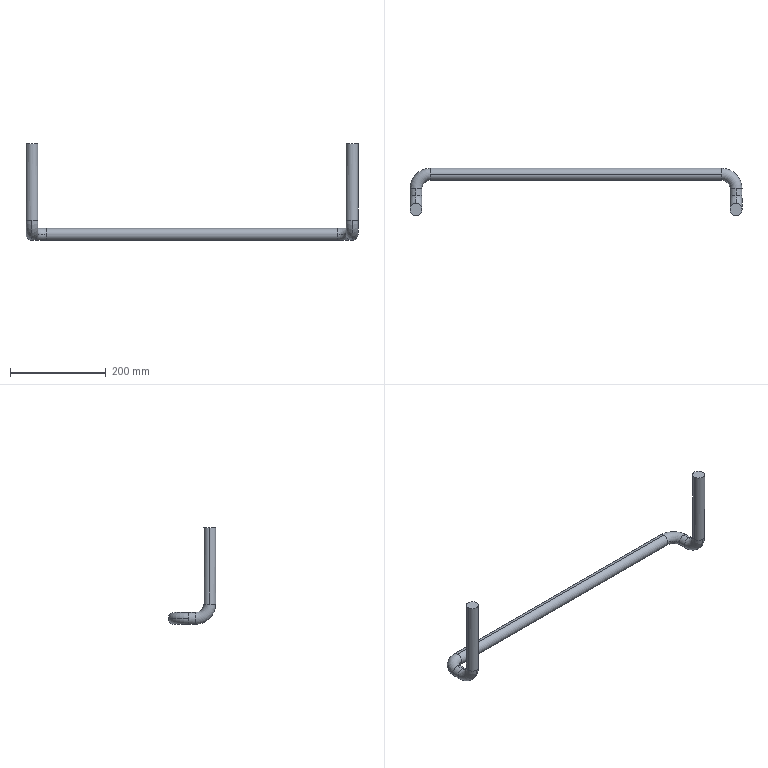Part | SolidWorks | features 3DProfileFeature 2, Sweep 1 | 1 solid | 20 faces | box 695 x 99.162 x 202.5 mm | volume 562944 mm3 | cylinder 10 | torus 8 | plane 2 | commonest cylinder face diameters 25 x10
STEP:
#1=CARTESIAN_POINT('',(-335.,-44.162,-12.5));
#2=VERTEX_POINT('',#1);
#3=CARTESIAN_POINT('',(-335.,-44.162,12.5));
#4=VERTEX_POINT('',#3);
#5=CARTESIAN_POINT('',(-335.,-44.162,0.));
#6=DIRECTION('',(0.,1.,0.));
#7=DIRECTION('',(-1.,0.,0.));
#8=AXIS2_PLACEMENT_3D('',#5,#6,#7);
#9=CIRCLE('',#8,12.5);
#10=EDGE_CURVE('',#2,#4,#9,.T.);
#11=ORIENTED_EDGE('',*,*,#10,.F.);
#12=CARTESIAN_POINT('',(-335.,-86.662,30.));
#13=VERTEX_POINT('',#12);
#14=CARTESIAN_POINT('',(-335.,-44.162,30.));
#15=DIRECTION('',(-1.,0.,0.));
#16=DIRECTION('',(0.,0.,1.));
#17=AXIS2_PLACEMENT_3D('',#14,#15,#16);
#18=CIRCLE('',#17,42.5);
#19=EDGE_CURVE('',#2,#13,#18,.T.);
#20=ORIENTED_EDGE('',*,*,#19,.T.);
#21=CARTESIAN_POINT('',(-347.5,-74.162,30.));
#22=VERTEX_POINT('',#21);
#23=CARTESIAN_POINT('',(-335.,-74.162,30.));
#24=DIRECTION('',(0.,0.,-1.));
#25=DIRECTION('',(-1.,0.,0.));
#26=AXIS2_PLACEMENT_3D('',#23,#24,#25);
#27=CIRCLE('',#26,12.5);
#28=EDGE_CURVE('',#13,#22,#27,.T.);
#29=ORIENTED_EDGE('',*,*,#28,.T.);
#30=CARTESIAN_POINT('',(-335.,-61.662,30.));
#31=VERTEX_POINT('',#30);
#32=CARTESIAN_POINT('',(-335.,-74.162,30.));
#33=DIRECTION('',(0.,0.,-1.));
#34=DIRECTION('',(-1.,0.,0.));
#35=AXIS2_PLACEMENT_3D('',#32,#33,#34);
#36=CIRCLE('',#35,12.5);
#37=EDGE_CURVE('',#22,#31,#36,.T.);
#38=ORIENTED_EDGE('',*,*,#37,.T.);
#39=CARTESIAN_POINT('',(-335.,-44.162,30.));
#40=DIRECTION('',(-1.,0.,0.));
#41=DIRECTION('',(0.,0.,1.));
#42=AXIS2_PLACEMENT_3D('',#39,#40,#41);
#43=CIRCLE('',#42,17.5);
#44=EDGE_CURVE('',#4,#31,#43,.T.);
#45=ORIENTED_EDGE('',*,*,#44,.F.);
#46=EDGE_LOOP('',(#11,#20,#29,#38,#45));
#47=FACE_OUTER_BOUND('',#46,.T.);
#48=CARTESIAN_POINT('',(-335.,-44.162,30.));
#49=DIRECTION('',(-1.,0.,0.));
#50=DIRECTION('',(0.,0.,1.));
#51=AXIS2_PLACEMENT_3D('',#48,#49,#50);
#52=TOROIDAL_SURFACE('',#51,30.,12.5);
#53=ADVANCED_FACE('',(#47),#52,.T.);
#54=CARTESIAN_POINT('',(-305.,12.5,0.));
#55=VERTEX_POINT('',#54);
#56=CARTESIAN_POINT('',(-305.,0.,12.5));
#57=VERTEX_POINT('',#56);
#58=CARTESIAN_POINT('',(-305.,0.,0.));
#59=DIRECTION('',(1.,0.,0.));
#60=DIRECTION('',(0.,1.,0.));
#61=AXIS2_PLACEMENT_3D('',#58,#59,#60);
#62=CIRCLE('',#61,12.5);
#63=EDGE_CURVE('',#55,#57,#62,.T.);
#64=ORIENTED_EDGE('',*,*,#63,.F.);
#65=CARTESIAN_POINT('',(-347.5,-30.,0.));
#66=VERTEX_POINT('',#65);
#67=CARTESIAN_POINT('',(-305.,-30.,0.));
#68=DIRECTION('',(0.,0.,1.));
#69=DIRECTION('',(1.,0.,0.));
#70=AXIS2_PLACEMENT_3D('',#67,#68,#69);
#71=CIRCLE('',#70,42.5);
#72=EDGE_CURVE('',#55,#66,#71,.T.);
#73=ORIENTED_EDGE('',*,*,#72,.T.);
#74=CARTESIAN_POINT('',(-335.,-30.,12.5));
#75=VERTEX_POINT('',#74);
#76=CARTESIAN_POINT('',(-335.,-30.,0.));
#77=DIRECTION('',(0.,1.,0.));
#78=DIRECTION('',(-1.,0.,0.));
#79=AXIS2_PLACEMENT_3D('',#76,#77,#78);
#80=CIRCLE('',#79,12.5);
#81=EDGE_CURVE('',#66,#75,#80,.T.);
#82=ORIENTED_EDGE('',*,*,#81,.T.);
#83=CARTESIAN_POINT('',(-322.5,-30.,0.));
#84=VERTEX_POINT('',#83);
#85=CARTESIAN_POINT('',(-335.,-30.,0.));
#86=DIRECTION('',(0.,1.,0.));
#87=DIRECTION('',(-1.,0.,0.));
#88=AXIS2_PLACEMENT_3D('',#85,#86,#87);
#89=CIRCLE('',#88,12.5);
#90=EDGE_CURVE('',#75,#84,#89,.T.);
#91=ORIENTED_EDGE('',*,*,#90,.T.);
#92=CARTESIAN_POINT('',(-305.,-12.5,0.));
#93=VERTEX_POINT('',#92);
#94=CARTESIAN_POINT('',(-305.,-30.,0.));
#95=DIRECTION('',(0.,0.,1.));
#96=DIRECTION('',(1.,0.,0.));
#97=AXIS2_PLACEMENT_3D('',#94,#95,#96);
#98=CIRCLE('',#97,17.5);
#99=EDGE_CURVE('',#93,#84,#98,.T.);
#100=ORIENTED_EDGE('',*,*,#99,.F.);
#101=CARTESIAN_POINT('',(-305.,0.,0.));
#102=DIRECTION('',(1.,0.,0.));
#103=DIRECTION('',(0.,1.,0.));
#104=AXIS2_PLACEMENT_3D('',#101,#102,#103);
#105=CIRCLE('',#104,12.5);
#106=EDGE_CURVE('',#57,#93,#105,.T.);
#107=ORIENTED_EDGE('',*,*,#106,.F.);
#108=EDGE_LOOP('',(#64,#73,#82,#91,#100,#107));
#109=FACE_OUTER_BOUND('',#108,.T.);
#110=CARTESIAN_POINT('',(-305.,-30.,0.));
#111=DIRECTION('',(0.,0.,1.));
#112=DIRECTION('',(1.,0.,0.));
#113=AXIS2_PLACEMENT_3D('',#110,#111,#112);
#114=TOROIDAL_SURFACE('',#113,30.,12.5);
#115=ADVANCED_FACE('',(#109),#114,.T.);
#116=CARTESIAN_POINT('',(347.5,-30.,0.));
#117=VERTEX_POINT('',#116);
#118=CARTESIAN_POINT('',(335.,-30.,12.5));
#119=VERTEX_POINT('',#118);
#120=CARTESIAN_POINT('',(335.,-30.,0.));
#121=DIRECTION('',(0.,-1.,0.));
#122=DIRECTION('',(1.,0.,0.));
#123=AXIS2_PLACEMENT_3D('',#120,#121,#122);
#124=CIRCLE('',#123,12.5);
#125=EDGE_CURVE('',#117,#119,#124,.T.);
#126=ORIENTED_EDGE('',*,*,#125,.F.);
#127=CARTESIAN_POINT('',(305.,12.5,0.));
#128=VERTEX_POINT('',#127);
#129=CARTESIAN_POINT('',(305.,-30.,0.));
#130=DIRECTION('',(0.,0.,1.));
#131=DIRECTION('',(1.,0.,0.));
#132=AXIS2_PLACEMENT_3D('',#129,#130,#131);
#133=CIRCLE('',#132,42.5);
#134=EDGE_CURVE('',#117,#128,#133,.T.);
#135=ORIENTED_EDGE('',*,*,#134,.T.);
#136=CARTESIAN_POINT('',(305.,0.,12.5));
#137=VERTEX_POINT('',#136);
#138=CARTESIAN_POINT('',(305.,0.,0.));
#139=DIRECTION('',(1.,0.,0.));
#140=DIRECTION('',(0.,1.,0.));
#141=AXIS2_PLACEMENT_3D('',#138,#139,#140);
#142=CIRCLE('',#141,12.5);
#143=EDGE_CURVE('',#128,#137,#142,.T.);
#144=ORIENTED_EDGE('',*,*,#143,.T.);
#145=CARTESIAN_POINT('',(305.,-12.5,0.));
#146=VERTEX_POINT('',#145);
#147=CARTESIAN_POINT('',(305.,0.,0.));
#148=DIRECTION('',(1.,0.,0.));
#149=DIRECTION('',(0.,1.,0.));
#150=AXIS2_PLACEMENT_3D('',#147,#148,#149);
#151=CIRCLE('',#150,12.5);
#152=EDGE_CURVE('',#137,#146,#151,.T.);
#153=ORIENTED_EDGE('',*,*,#152,.T.);
#154=CARTESIAN_POINT('',(322.5,-30.,0.));
#155=VERTEX_POINT('',#154);
#156=CARTESIAN_POINT('',(305.,-30.,0.));
#157=DIRECTION('',(0.,0.,1.));
#158=DIRECTION('',(1.,0.,0.));
#159=AXIS2_PLACEMENT_3D('',#156,#157,#158);
#160=CIRCLE('',#159,17.5);
#161=EDGE_CURVE('',#155,#146,#160,.T.);
#162=ORIENTED_EDGE('',*,*,#161,.F.);
#163=CARTESIAN_POINT('',(335.,-30.,0.));
#164=DIRECTION('',(0.,-1.,0.));
#165=DIRECTION('',(1.,0.,0.));
#166=AXIS2_PLACEMENT_3D('',#163,#164,#165);
#167=CIRCLE('',#166,12.5);
#168=EDGE_CURVE('',#119,#155,#167,.T.);
#169=ORIENTED_EDGE('',*,*,#168,.F.);
#170=EDGE_LOOP('',(#126,#135,#144,#153,#162,#169));
#171=FACE_OUTER_BOUND('',#170,.T.);
#172=CARTESIAN_POINT('',(305.,-30.,0.));
#173=DIRECTION('',(0.,0.,1.));
#174=DIRECTION('',(1.,0.,0.));
#175=AXIS2_PLACEMENT_3D('',#172,#173,#174);
#176=TOROIDAL_SURFACE('',#175,30.,12.5);
#177=ADVANCED_FACE('',(#171),#176,.T.);
#178=CARTESIAN_POINT('',(335.,-86.662,30.));
#179=VERTEX_POINT('',#178);
#180=CARTESIAN_POINT('',(347.5,-74.162,30.));
#181=VERTEX_POINT('',#180);
#182=CARTESIAN_POINT('',(335.,-74.162,30.));
#183=DIRECTION('',(0.,0.,1.));
#184=DIRECTION('',(1.,0.,0.));
#185=AXIS2_PLACEMENT_3D('',#182,#183,#184);
#186=CIRCLE('',#185,12.5);
#187=EDGE_CURVE('',#179,#181,#186,.T.);
#188=ORIENTED_EDGE('',*,*,#187,.F.);
#189=CARTESIAN_POINT('',(335.,-44.162,-12.5));
#190=VERTEX_POINT('',#189);
#191=CARTESIAN_POINT('',(335.,-44.162,30.));
#192=DIRECTION('',(1.,0.,0.));
#193=DIRECTION('',(0.,0.,-1.));
#194=AXIS2_PLACEMENT_3D('',#191,#192,#193);
#195=CIRCLE('',#194,42.5);
#196=EDGE_CURVE('',#179,#190,#195,.T.);
#197=ORIENTED_EDGE('',*,*,#196,.T.);
#198=CARTESIAN_POINT('',(335.,-44.162,12.5));
#199=VERTEX_POINT('',#198);
#200=CARTESIAN_POINT('',(335.,-44.162,0.));
#201=DIRECTION('',(0.,-1.,0.));
#202=DIRECTION('',(1.,0.,0.));
#203=AXIS2_PLACEMENT_3D('',#200,#201,#202);
#204=CIRCLE('',#203,12.5);
#205=EDGE_CURVE('',#190,#199,#204,.T.);
#206=ORIENTED_EDGE('',*,*,#205,.T.);
#207=CARTESIAN_POINT('',(335.,-61.662,30.));
#208=VERTEX_POINT('',#207);
#209=CARTESIAN_POINT('',(335.,-44.162,30.));
#210=DIRECTION('',(1.,0.,0.));
#211=DIRECTION('',(0.,0.,-1.));
#212=AXIS2_PLACEMENT_3D('',#209,#210,#211);
#213=CIRCLE('',#212,17.5);
#214=EDGE_CURVE('',#208,#199,#213,.T.);
#215=ORIENTED_EDGE('',*,*,#214,.F.);
#216=CARTESIAN_POINT('',(335.,-74.162,30.));
#217=DIRECTION('',(0.,0.,1.));
#218=DIRECTION('',(1.,0.,0.));
#219=AXIS2_PLACEMENT_3D('',#216,#217,#218);
#220=CIRCLE('',#219,12.5);
#221=EDGE_CURVE('',#181,#208,#220,.T.);
#222=ORIENTED_EDGE('',*,*,#221,.F.);
#223=EDGE_LOOP('',(#188,#197,#206,#215,#222));
#224=FACE_OUTER_BOUND('',#223,.T.);
#225=CARTESIAN_POINT('',(335.,-44.162,30.));
#226=DIRECTION('',(1.,0.,0.));
#227=DIRECTION('',(0.,0.,-1.));
#228=AXIS2_PLACEMENT_3D('',#225,#226,#227);
#229=TOROIDAL_SURFACE('',#228,30.,12.5);
#230=ADVANCED_FACE('',(#224),#229,.T.);
#231=ORIENTED_EDGE('',*,*,#37,.F.);
#232=CARTESIAN_POINT('',(-347.5,-74.162,190.));
#233=VERTEX_POINT('',#232);
#234=CARTESIAN_POINT('',(-347.5,-74.162,30.));
#235=DIRECTION('',(0.,0.,1.));
#236=VECTOR('',#235,1000.);
#237=LINE('',#234,#236);
#238=EDGE_CURVE('',#22,#233,#237,.T.);
#239=ORIENTED_EDGE('',*,*,#238,.T.);
#240=CARTESIAN_POINT('',(-322.5,-74.162,190.));
#241=VERTEX_POINT('',#240);
#242=CARTESIAN_POINT('',(-335.,-74.162,190.));
#243=DIRECTION('',(0.,0.,-1.));
#244=DIRECTION('',(-1.,0.,0.));
#245=AXIS2_PLACEMENT_3D('',#242,#243,#244);
#246=CIRCLE('',#245,12.5);
#247=EDGE_CURVE('',#233,#241,#246,.T.);
#248=ORIENTED_EDGE('',*,*,#247,.T.);
#249=CARTESIAN_POINT('',(-322.5,-74.162,30.));
#250=VERTEX_POINT('',#249);
#251=CARTESIAN_POINT('',(-322.5,-74.162,30.));
#252=DIRECTION('',(0.,0.,1.));
#253=VECTOR('',#252,1000.);
#254=LINE('',#251,#253);
#255=EDGE_CURVE('',#250,#241,#254,.T.);
#256=ORIENTED_EDGE('',*,*,#255,.F.);
#257=CARTESIAN_POINT('',(-335.,-74.162,30.));
#258=DIRECTION('',(0.,0.,-1.));
#259=DIRECTION('',(-1.,0.,0.));
#260=AXIS2_PLACEMENT_3D('',#257,#258,#259);
#261=CIRCLE('',#260,12.5);
#262=EDGE_CURVE('',#31,#250,#261,.T.);
#263=ORIENTED_EDGE('',*,*,#262,.F.);
#264=EDGE_LOOP('',(#231,#239,#248,#256,#263));
#265=FACE_OUTER_BOUND('',#264,.T.);
#266=CARTESIAN_POINT('',(-335.,-74.162,30.));
#267=DIRECTION('',(0.,0.,1.));
#268=DIRECTION('',(1.,0.,0.));
#269=AXIS2_PLACEMENT_3D('',#266,#267,#268);
#270=CYLINDRICAL_SURFACE('',#269,12.5);
#271=ADVANCED_FACE('',(#265),#270,.T.);
#272=ORIENTED_EDGE('',*,*,#90,.F.);
#273=CARTESIAN_POINT('',(-335.,-30.,12.5));
#274=DIRECTION('',(0.,-1.,0.));
#275=VECTOR('',#274,1000.);
#276=LINE('',#273,#275);
#277=EDGE_CURVE('',#75,#4,#276,.T.);
#278=ORIENTED_EDGE('',*,*,#277,.T.);
#279=CARTESIAN_POINT('',(-335.,-44.162,0.));
#280=DIRECTION('',(0.,1.,0.));
#281=DIRECTION('',(-1.,0.,0.));
#282=AXIS2_PLACEMENT_3D('',#279,#280,#281);
#283=CIRCLE('',#282,12.5);
#284=EDGE_CURVE('',#4,#2,#283,.T.);
#285=ORIENTED_EDGE('',*,*,#284,.T.);
#286=CARTESIAN_POINT('',(-335.,-30.,-12.5));
#287=VERTEX_POINT('',#286);
#288=CARTESIAN_POINT('',(-335.,-30.,-12.5));
#289=DIRECTION('',(0.,-1.,0.));
#290=VECTOR('',#289,1000.);
#291=LINE('',#288,#290);
#292=EDGE_CURVE('',#287,#2,#291,.T.);
#293=ORIENTED_EDGE('',*,*,#292,.F.);
#294=CARTESIAN_POINT('',(-335.,-30.,0.));
#295=DIRECTION('',(0.,1.,0.));
#296=DIRECTION('',(-1.,0.,0.));
#297=AXIS2_PLACEMENT_3D('',#294,#295,#296);
#298=CIRCLE('',#297,12.5);
#299=EDGE_CURVE('',#84,#287,#298,.T.);
#300=ORIENTED_EDGE('',*,*,#299,.F.);
#301=EDGE_LOOP('',(#272,#278,#285,#293,#300));
#302=FACE_OUTER_BOUND('',#301,.T.);
#303=CARTESIAN_POINT('',(-335.,-30.,0.));
#304=DIRECTION('',(0.,-1.,0.));
#305=DIRECTION('',(0.,0.,-1.));
#306=AXIS2_PLACEMENT_3D('',#303,#304,#305);
#307=CYLINDRICAL_SURFACE('',#306,12.5);
#308=ADVANCED_FACE('',(#302),#307,.T.);
#309=CARTESIAN_POINT('',(305.,0.,-12.5));
#310=VERTEX_POINT('',#309);
#311=CARTESIAN_POINT('',(305.,0.,0.));
#312=DIRECTION('',(1.,0.,0.));
#313=DIRECTION('',(0.,1.,0.));
#314=AXIS2_PLACEMENT_3D('',#311,#312,#313);
#315=CIRCLE('',#314,12.5);
#316=EDGE_CURVE('',#310,#128,#315,.T.);
#317=ORIENTED_EDGE('',*,*,#316,.F.);
#318=CARTESIAN_POINT('',(-305.,0.,-12.5));
#319=VERTEX_POINT('',#318);
#320=CARTESIAN_POINT('',(305.,0.,-12.5));
#321=DIRECTION('',(-1.,0.,0.));
#322=VECTOR('',#321,1000.);
#323=LINE('',#320,#322);
#324=EDGE_CURVE('',#310,#319,#323,.T.);
#325=ORIENTED_EDGE('',*,*,#324,.T.);
#326=CARTESIAN_POINT('',(-305.,0.,0.));
#327=DIRECTION('',(1.,0.,0.));
#328=DIRECTION('',(0.,1.,0.));
#329=AXIS2_PLACEMENT_3D('',#326,#327,#328);
#330=CIRCLE('',#329,12.5);
#331=EDGE_CURVE('',#319,#55,#330,.T.);
#332=ORIENTED_EDGE('',*,*,#331,.T.);
#333=ORIENTED_EDGE('',*,*,#63,.T.);
#334=CARTESIAN_POINT('',(305.,0.,12.5));
#335=DIRECTION('',(-1.,0.,0.));
#336=VECTOR('',#335,1000.);
#337=LINE('',#334,#336);
#338=EDGE_CURVE('',#137,#57,#337,.T.);
#339=ORIENTED_EDGE('',*,*,#338,.F.);
#340=ORIENTED_EDGE('',*,*,#143,.F.);
#341=EDGE_LOOP('',(#317,#325,#332,#333,#339,#340));
#342=FACE_OUTER_BOUND('',#341,.T.);
#343=CARTESIAN_POINT('',(305.,0.,0.));
#344=DIRECTION('',(-1.,0.,0.));
#345=DIRECTION('',(0.,0.,1.));
#346=AXIS2_PLACEMENT_3D('',#343,#344,#345);
#347=CYLINDRICAL_SURFACE('',#346,12.5);
#348=ADVANCED_FACE('',(#342),#347,.T.);
#349=ORIENTED_EDGE('',*,*,#205,.F.);
#350=CARTESIAN_POINT('',(335.,-30.,-12.5));
#351=VERTEX_POINT('',#350);
#352=CARTESIAN_POINT('',(335.,-44.162,-12.5));
#353=DIRECTION('',(0.,1.,0.));
#354=VECTOR('',#353,1000.);
#355=LINE('',#352,#354);
#356=EDGE_CURVE('',#190,#351,#355,.T.);
#357=ORIENTED_EDGE('',*,*,#356,.T.);
#358=CARTESIAN_POINT('',(335.,-30.,0.));
#359=DIRECTION('',(0.,-1.,0.));
#360=DIRECTION('',(1.,0.,0.));
#361=AXIS2_PLACEMENT_3D('',#358,#359,#360);
#362=CIRCLE('',#361,12.5);
#363=EDGE_CURVE('',#351,#117,#362,.T.);
#364=ORIENTED_EDGE('',*,*,#363,.T.);
#365=ORIENTED_EDGE('',*,*,#125,.T.);
#366=CARTESIAN_POINT('',(335.,-44.162,12.5));
#367=DIRECTION('',(0.,1.,0.));
#368=VECTOR('',#367,1000.);
#369=LINE('',#366,#368);
#370=EDGE_CURVE('',#199,#119,#369,.T.);
#371=ORIENTED_EDGE('',*,*,#370,.F.);
#372=EDGE_LOOP('',(#349,#357,#364,#365,#371));
#373=FACE_OUTER_BOUND('',#372,.T.);
#374=CARTESIAN_POINT('',(335.,-44.162,0.));
#375=DIRECTION('',(0.,1.,0.));
#376=DIRECTION('',(0.,0.,1.));
#377=AXIS2_PLACEMENT_3D('',#374,#375,#376);
#378=CYLINDRICAL_SURFACE('',#377,12.5);
#379=ADVANCED_FACE('',(#373),#378,.T.);
#380=CARTESIAN_POINT('',(347.5,-74.162,190.));
#381=VERTEX_POINT('',#380);
#382=CARTESIAN_POINT('',(322.5,-74.162,190.));
#383=VERTEX_POINT('',#382);
#384=CARTESIAN_POINT('',(335.,-74.162,190.));
#385=DIRECTION('',(0.,0.,1.));
#386=DIRECTION('',(1.,0.,0.));
#387=AXIS2_PLACEMENT_3D('',#384,#385,#386);
#388=CIRCLE('',#387,12.5);
#389=EDGE_CURVE('',#381,#383,#388,.T.);
#390=ORIENTED_EDGE('',*,*,#389,.F.);
#391=CARTESIAN_POINT('',(347.5,-74.162,190.));
#392=DIRECTION('',(0.,0.,-1.));
#393=VECTOR('',#392,1000.);
#394=LINE('',#391,#393);
#395=EDGE_CURVE('',#381,#181,#394,.T.);
#396=ORIENTED_EDGE('',*,*,#395,.T.);
#397=ORIENTED_EDGE('',*,*,#221,.T.);
#398=CARTESIAN_POINT('',(322.5,-74.162,30.));
#399=VERTEX_POINT('',#398);
#400=CARTESIAN_POINT('',(335.,-74.162,30.));
#401=DIRECTION('',(0.,0.,1.));
#402=DIRECTION('',(1.,0.,0.));
#403=AXIS2_PLACEMENT_3D('',#400,#401,#402);
#404=CIRCLE('',#403,12.5);
#405=EDGE_CURVE('',#208,#399,#404,.T.);
#406=ORIENTED_EDGE('',*,*,#405,.T.);
#407=CARTESIAN_POINT('',(322.5,-74.162,190.));
#408=DIRECTION('',(0.,0.,-1.));
#409=VECTOR('',#408,1000.);
#410=LINE('',#407,#409);
#411=EDGE_CURVE('',#383,#399,#410,.T.);
#412=ORIENTED_EDGE('',*,*,#411,.F.);
#413=EDGE_LOOP('',(#390,#396,#397,#406,#412));
#414=FACE_OUTER_BOUND('',#413,.T.);
#415=CARTESIAN_POINT('',(335.,-74.162,190.));
#416=DIRECTION('',(0.,0.,-1.));
#417=DIRECTION('',(-1.,0.,0.));
#418=AXIS2_PLACEMENT_3D('',#415,#416,#417);
#419=CYLINDRICAL_SURFACE('',#418,12.5);
#420=ADVANCED_FACE('',(#414),#419,.T.);
#421=ORIENTED_EDGE('',*,*,#238,.F.);
#422=ORIENTED_EDGE('',*,*,#28,.F.);
#423=CARTESIAN_POINT('',(-335.,-74.162,30.));
#424=DIRECTION('',(0.,0.,-1.));
#425=DIRECTION('',(-1.,0.,0.));
#426=AXIS2_PLACEMENT_3D('',#423,#424,#425);
#427=CIRCLE('',#426,12.5);
#428=EDGE_CURVE('',#250,#13,#427,.T.);
#429=ORIENTED_EDGE('',*,*,#428,.F.);
#430=ORIENTED_EDGE('',*,*,#255,.T.);
#431=CARTESIAN_POINT('',(-335.,-74.162,190.));
#432=DIRECTION('',(0.,0.,-1.));
#433=DIRECTION('',(-1.,0.,0.));
#434=AXIS2_PLACEMENT_3D('',#431,#432,#433);
#435=CIRCLE('',#434,12.5);
#436=EDGE_CURVE('',#241,#233,#435,.T.);
#437=ORIENTED_EDGE('',*,*,#436,.T.);
#438=EDGE_LOOP('',(#421,#422,#429,#430,#437));
#439=FACE_OUTER_BOUND('',#438,.T.);
#440=CARTESIAN_POINT('',(-335.,-74.162,30.));
#441=DIRECTION('',(0.,0.,1.));
#442=DIRECTION('',(1.,0.,0.));
#443=AXIS2_PLACEMENT_3D('',#440,#441,#442);
#444=CYLINDRICAL_SURFACE('',#443,12.5);
#445=ADVANCED_FACE('',(#439),#444,.T.);
#446=ORIENTED_EDGE('',*,*,#19,.F.);
#447=ORIENTED_EDGE('',*,*,#284,.F.);
#448=ORIENTED_EDGE('',*,*,#44,.T.);
#449=ORIENTED_EDGE('',*,*,#262,.T.);
#450=ORIENTED_EDGE('',*,*,#428,.T.);
#451=EDGE_LOOP('',(#446,#447,#448,#449,#450));
#452=FACE_OUTER_BOUND('',#451,.T.);
#453=CARTESIAN_POINT('',(-335.,-44.162,30.));
#454=DIRECTION('',(-1.,0.,0.));
#455=DIRECTION('',(0.,0.,1.));
#456=AXIS2_PLACEMENT_3D('',#453,#454,#455);
#457=TOROIDAL_SURFACE('',#456,30.,12.5);
#458=ADVANCED_FACE('',(#452),#457,.T.);
#459=ORIENTED_EDGE('',*,*,#277,.F.);
#460=ORIENTED_EDGE('',*,*,#81,.F.);
#461=CARTESIAN_POINT('',(-335.,-30.,0.));
#462=DIRECTION('',(0.,1.,0.));
#463=DIRECTION('',(-1.,0.,0.));
#464=AXIS2_PLACEMENT_3D('',#461,#462,#463);
#465=CIRCLE('',#464,12.5);
#466=EDGE_CURVE('',#287,#66,#465,.T.);
#467=ORIENTED_EDGE('',*,*,#466,.F.);
#468=ORIENTED_EDGE('',*,*,#292,.T.);
#469=ORIENTED_EDGE('',*,*,#10,.T.);
#470=EDGE_LOOP('',(#459,#460,#467,#468,#469));
#471=FACE_OUTER_BOUND('',#470,.T.);
#472=CARTESIAN_POINT('',(-335.,-30.,0.));
#473=DIRECTION('',(0.,-1.,0.));
#474=DIRECTION('',(0.,0.,-1.));
#475=AXIS2_PLACEMENT_3D('',#472,#473,#474);
#476=CYLINDRICAL_SURFACE('',#475,12.5);
#477=ADVANCED_FACE('',(#471),#476,.T.);
#478=ORIENTED_EDGE('',*,*,#72,.F.);
#479=ORIENTED_EDGE('',*,*,#331,.F.);
#480=CARTESIAN_POINT('',(-305.,0.,0.));
#481=DIRECTION('',(1.,0.,0.));
#482=DIRECTION('',(0.,1.,0.));
#483=AXIS2_PLACEMENT_3D('',#480,#481,#482);
#484=CIRCLE('',#483,12.5);
#485=EDGE_CURVE('',#93,#319,#484,.T.);
#486=ORIENTED_EDGE('',*,*,#485,.F.);
#487=ORIENTED_EDGE('',*,*,#99,.T.);
#488=ORIENTED_EDGE('',*,*,#299,.T.);
#489=ORIENTED_EDGE('',*,*,#466,.T.);
#490=EDGE_LOOP('',(#478,#479,#486,#487,#488,#489));
#491=FACE_OUTER_BOUND('',#490,.T.);
#492=CARTESIAN_POINT('',(-305.,-30.,0.));
#493=DIRECTION('',(0.,0.,1.));
#494=DIRECTION('',(1.,0.,0.));
#495=AXIS2_PLACEMENT_3D('',#492,#493,#494);
#496=TOROIDAL_SURFACE('',#495,30.,12.5);
#497=ADVANCED_FACE('',(#491),#496,.T.);
#498=ORIENTED_EDGE('',*,*,#324,.F.);
#499=CARTESIAN_POINT('',(305.,0.,0.));
#500=DIRECTION('',(1.,0.,0.));
#501=DIRECTION('',(0.,1.,0.));
#502=AXIS2_PLACEMENT_3D('',#499,#500,#501);
#503=CIRCLE('',#502,12.5);
#504=EDGE_CURVE('',#146,#310,#503,.T.);
#505=ORIENTED_EDGE('',*,*,#504,.F.);
#506=ORIENTED_EDGE('',*,*,#152,.F.);
#507=ORIENTED_EDGE('',*,*,#338,.T.);
#508=ORIENTED_EDGE('',*,*,#106,.T.);
#509=ORIENTED_EDGE('',*,*,#485,.T.);
#510=EDGE_LOOP('',(#498,#505,#506,#507,#508,#509));
#511=FACE_OUTER_BOUND('',#510,.T.);
#512=CARTESIAN_POINT('',(305.,0.,0.));
#513=DIRECTION('',(-1.,0.,0.));
#514=DIRECTION('',(0.,0.,1.));
#515=AXIS2_PLACEMENT_3D('',#512,#513,#514);
#516=CYLINDRICAL_SURFACE('',#515,12.5);
#517=ADVANCED_FACE('',(#511),#516,.T.);
#518=ORIENTED_EDGE('',*,*,#134,.F.);
#519=ORIENTED_EDGE('',*,*,#363,.F.);
#520=CARTESIAN_POINT('',(335.,-30.,0.));
#521=DIRECTION('',(0.,-1.,0.));
#522=DIRECTION('',(1.,0.,0.));
#523=AXIS2_PLACEMENT_3D('',#520,#521,#522);
#524=CIRCLE('',#523,12.5);
#525=EDGE_CURVE('',#155,#351,#524,.T.);
#526=ORIENTED_EDGE('',*,*,#525,.F.);
#527=ORIENTED_EDGE('',*,*,#161,.T.);
#528=ORIENTED_EDGE('',*,*,#504,.T.);
#529=ORIENTED_EDGE('',*,*,#316,.T.);
#530=EDGE_LOOP('',(#518,#519,#526,#527,#528,#529));
#531=FACE_OUTER_BOUND('',#530,.T.);
#532=CARTESIAN_POINT('',(305.,-30.,0.));
#533=DIRECTION('',(0.,0.,1.));
#534=DIRECTION('',(1.,0.,0.));
#535=AXIS2_PLACEMENT_3D('',#532,#533,#534);
#536=TOROIDAL_SURFACE('',#535,30.,12.5);
#537=ADVANCED_FACE('',(#531),#536,.T.);
#538=ORIENTED_EDGE('',*,*,#356,.F.);
#539=CARTESIAN_POINT('',(335.,-44.162,0.));
#540=DIRECTION('',(0.,-1.,0.));
#541=DIRECTION('',(1.,0.,0.));
#542=AXIS2_PLACEMENT_3D('',#539,#540,#541);
#543=CIRCLE('',#542,12.5);
#544=EDGE_CURVE('',#199,#190,#543,.T.);
#545=ORIENTED_EDGE('',*,*,#544,.F.);
#546=ORIENTED_EDGE('',*,*,#370,.T.);
#547=ORIENTED_EDGE('',*,*,#168,.T.);
#548=ORIENTED_EDGE('',*,*,#525,.T.);
#549=EDGE_LOOP('',(#538,#545,#546,#547,#548));
#550=FACE_OUTER_BOUND('',#549,.T.);
#551=CARTESIAN_POINT('',(335.,-44.162,0.));
#552=DIRECTION('',(0.,1.,0.));
#553=DIRECTION('',(0.,0.,1.));
#554=AXIS2_PLACEMENT_3D('',#551,#552,#553);
#555=CYLINDRICAL_SURFACE('',#554,12.5);
#556=ADVANCED_FACE('',(#550),#555,.T.);
#557=ORIENTED_EDGE('',*,*,#196,.F.);
#558=CARTESIAN_POINT('',(335.,-74.162,30.));
#559=DIRECTION('',(0.,0.,1.));
#560=DIRECTION('',(1.,0.,0.));
#561=AXIS2_PLACEMENT_3D('',#558,#559,#560);
#562=CIRCLE('',#561,12.5);
#563=EDGE_CURVE('',#399,#179,#562,.T.);
#564=ORIENTED_EDGE('',*,*,#563,.F.);
#565=ORIENTED_EDGE('',*,*,#405,.F.);
#566=ORIENTED_EDGE('',*,*,#214,.T.);
#567=ORIENTED_EDGE('',*,*,#544,.T.);
#568=EDGE_LOOP('',(#557,#564,#565,#566,#567));
#569=FACE_OUTER_BOUND('',#568,.T.);
#570=CARTESIAN_POINT('',(335.,-44.162,30.));
#571=DIRECTION('',(1.,0.,0.));
#572=DIRECTION('',(0.,0.,-1.));
#573=AXIS2_PLACEMENT_3D('',#570,#571,#572);
#574=TOROIDAL_SURFACE('',#573,30.,12.5);
#575=ADVANCED_FACE('',(#569),#574,.T.);
#576=ORIENTED_EDGE('',*,*,#395,.F.);
#577=CARTESIAN_POINT('',(335.,-74.162,190.));
#578=DIRECTION('',(0.,0.,1.));
#579=DIRECTION('',(1.,0.,0.));
#580=AXIS2_PLACEMENT_3D('',#577,#578,#579);
#581=CIRCLE('',#580,12.5);
#582=EDGE_CURVE('',#383,#381,#581,.T.);
#583=ORIENTED_EDGE('',*,*,#582,.F.);
#584=ORIENTED_EDGE('',*,*,#411,.T.);
#585=ORIENTED_EDGE('',*,*,#563,.T.);
#586=ORIENTED_EDGE('',*,*,#187,.T.);
#587=EDGE_LOOP('',(#576,#583,#584,#585,#586));
#588=FACE_OUTER_BOUND('',#587,.T.);
#589=CARTESIAN_POINT('',(335.,-74.162,190.));
#590=DIRECTION('',(0.,0.,-1.));
#591=DIRECTION('',(-1.,0.,0.));
#592=AXIS2_PLACEMENT_3D('',#589,#590,#591);
#593=CYLINDRICAL_SURFACE('',#592,12.5);
#594=ADVANCED_FACE('',(#588),#593,.T.);
#595=ORIENTED_EDGE('',*,*,#436,.F.);
#596=ORIENTED_EDGE('',*,*,#247,.F.);
#597=EDGE_LOOP('',(#595,#596));
#598=FACE_OUTER_BOUND('',#597,.T.);
#599=CARTESIAN_POINT('',(-335.,-74.162,190.));
#600=DIRECTION('',(0.,0.,-1.));
#601=DIRECTION('',(-1.,0.,0.));
#602=AXIS2_PLACEMENT_3D('',#599,#600,#601);
#603=PLANE('',#602);
#604=ADVANCED_FACE('',(#598),#603,.F.);
#605=ORIENTED_EDGE('',*,*,#582,.T.);
#606=ORIENTED_EDGE('',*,*,#389,.T.);
#607=EDGE_LOOP('',(#605,#606));
#608=FACE_OUTER_BOUND('',#607,.T.);
#609=CARTESIAN_POINT('',(335.,-74.162,190.));
#610=DIRECTION('',(0.,0.,1.));
#611=DIRECTION('',(1.,0.,0.));
#612=AXIS2_PLACEMENT_3D('',#609,#610,#611);
#613=PLANE('',#612);
#614=ADVANCED_FACE('',(#608),#613,.T.);
#615=CLOSED_SHELL('',(#53,#115,#177,#230,#271,#308,#348,#379,#420,#445,#458,#477,#497,#517,#537,#556,#575,#594,#604,#614));
#616=MANIFOLD_SOLID_BREP('',#615);
#617=CARTESIAN_POINT('',(0.,0.,0.));
#618=DIRECTION('',(0.,0.,1.));
#619=DIRECTION('',(1.,0.,0.));
#620=AXIS2_PLACEMENT_3D('',#617,#618,#619);
#621=(LENGTH_UNIT()NAMED_UNIT(*)SI_UNIT(.MILLI.,.METRE.));
#622=UNCERTAINTY_MEASURE_WITH_UNIT(LENGTH_MEASURE(0.00001),#621,'','');
#623=(NAMED_UNIT(*)PLANE_ANGLE_UNIT()SI_UNIT($,.RADIAN.));
#624=(NAMED_UNIT(*)SI_UNIT($,.STERADIAN.)SOLID_ANGLE_UNIT());
#625=(GEOMETRIC_REPRESENTATION_CONTEXT(3)GLOBAL_UNCERTAINTY_ASSIGNED_CONTEXT((#622))GLOBAL_UNIT_ASSIGNED_CONTEXT((#621,#623,#624))REPRESENTATION_CONTEXT('',''));
#626=ADVANCED_BREP_SHAPE_REPRESENTATION('',(#616,#620),#625);